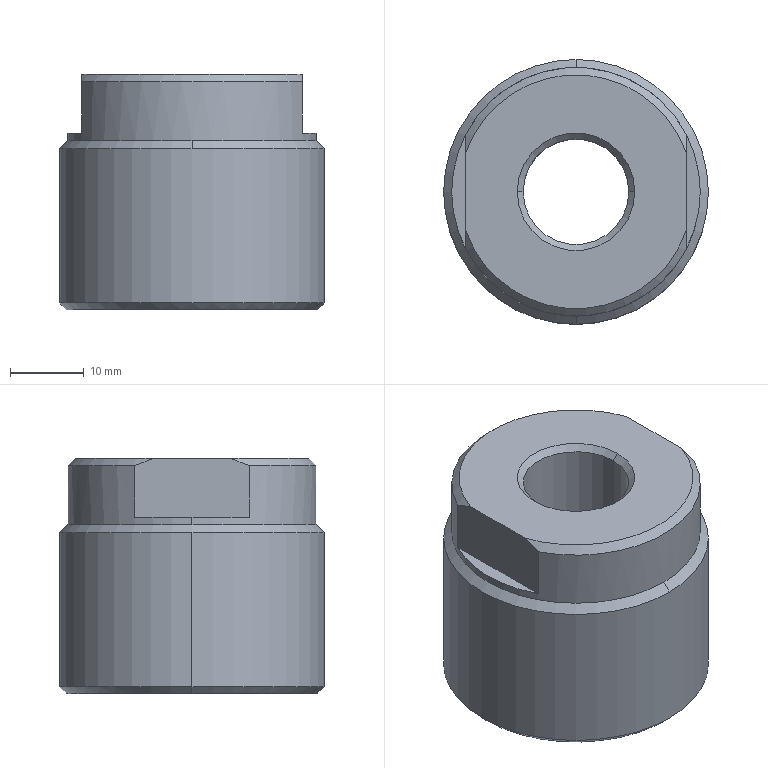Part | SolidWorks | features BaseBody 1 | 1 solid | 25 faces | box 36 x 36 x 32 mm | volume 25281 mm3 | cone 10 | cylinder 8 | plane 7 | commonest cylinder face diameters 14.376 x2 16.5 x2 33.8 x2 36 x2
STEP:
#1=CARTESIAN_POINT('',(18.,0.,0.92));
#2=VERTEX_POINT('',#1);
#3=CARTESIAN_POINT('',(-18.,0.,0.92));
#4=VERTEX_POINT('',#3);
#5=CARTESIAN_POINT('',(0.,0.,0.92));
#6=DIRECTION('',(0.,0.,1.));
#7=DIRECTION('',(1.,0.,0.));
#8=AXIS2_PLACEMENT_3D('',#5,#6,#7);
#9=CIRCLE('',#8,18.);
#10=EDGE_CURVE('',#2,#4,#9,.T.);
#11=ORIENTED_EDGE('',*,*,#10,.T.);
#12=CARTESIAN_POINT('',(-18.,0.,21.9));
#13=VERTEX_POINT('',#12);
#14=CARTESIAN_POINT('',(-18.,0.,0.));
#15=DIRECTION('',(0.,0.,1.));
#16=VECTOR('',#15,1000.);
#17=LINE('',#14,#16);
#18=EDGE_CURVE('',#4,#13,#17,.T.);
#19=ORIENTED_EDGE('',*,*,#18,.T.);
#20=CARTESIAN_POINT('',(0.,18.,21.9));
#21=VERTEX_POINT('',#20);
#22=CARTESIAN_POINT('',(0.,0.,21.9));
#23=DIRECTION('',(0.,0.,-1.));
#24=DIRECTION('',(1.,0.,0.));
#25=AXIS2_PLACEMENT_3D('',#22,#23,#24);
#26=CIRCLE('',#25,18.);
#27=EDGE_CURVE('',#13,#21,#26,.T.);
#28=ORIENTED_EDGE('',*,*,#27,.T.);
#29=CARTESIAN_POINT('',(18.,0.,21.9));
#30=VERTEX_POINT('',#29);
#31=CARTESIAN_POINT('',(0.,0.,21.9));
#32=DIRECTION('',(0.,0.,-1.));
#33=DIRECTION('',(1.,0.,0.));
#34=AXIS2_PLACEMENT_3D('',#31,#32,#33);
#35=CIRCLE('',#34,18.);
#36=EDGE_CURVE('',#21,#30,#35,.T.);
#37=ORIENTED_EDGE('',*,*,#36,.T.);
#38=CARTESIAN_POINT('',(18.,0.,0.));
#39=DIRECTION('',(0.,0.,1.));
#40=VECTOR('',#39,1000.);
#41=LINE('',#38,#40);
#42=EDGE_CURVE('',#2,#30,#41,.T.);
#43=ORIENTED_EDGE('',*,*,#42,.F.);
#44=EDGE_LOOP('',(#11,#19,#28,#37,#43));
#45=FACE_OUTER_BOUND('',#44,.T.);
#46=CARTESIAN_POINT('',(0.,0.,0.));
#47=DIRECTION('',(0.,0.,1.));
#48=DIRECTION('',(1.,0.,0.));
#49=AXIS2_PLACEMENT_3D('',#46,#47,#48);
#50=CYLINDRICAL_SURFACE('',#49,18.);
#51=ADVANCED_FACE('',(#45),#50,.T.);
#52=CARTESIAN_POINT('',(17.08,0.,0.));
#53=VERTEX_POINT('',#52);
#54=CARTESIAN_POINT('',(-17.08,0.,0.));
#55=VERTEX_POINT('',#54);
#56=CARTESIAN_POINT('',(0.,0.,0.));
#57=DIRECTION('',(0.,0.,1.));
#58=DIRECTION('',(1.,0.,0.));
#59=AXIS2_PLACEMENT_3D('',#56,#57,#58);
#60=CIRCLE('',#59,17.08);
#61=EDGE_CURVE('',#53,#55,#60,.T.);
#62=ORIENTED_EDGE('',*,*,#61,.T.);
#63=CARTESIAN_POINT('',(-18.,0.,0.92));
#64=DIRECTION('',(-0.7071,0.,0.7071));
#65=VECTOR('',#64,1000.);
#66=LINE('',#63,#65);
#67=EDGE_CURVE('',#55,#4,#66,.T.);
#68=ORIENTED_EDGE('',*,*,#67,.T.);
#69=ORIENTED_EDGE('',*,*,#10,.F.);
#70=CARTESIAN_POINT('',(18.,0.,0.92));
#71=DIRECTION('',(0.7071,0.,0.7071));
#72=VECTOR('',#71,1000.);
#73=LINE('',#70,#72);
#74=EDGE_CURVE('',#53,#2,#73,.T.);
#75=ORIENTED_EDGE('',*,*,#74,.F.);
#76=EDGE_LOOP('',(#62,#68,#69,#75));
#77=FACE_OUTER_BOUND('',#76,.T.);
#78=CARTESIAN_POINT('',(0.,0.,0.92));
#79=DIRECTION('',(0.,0.,1.));
#80=DIRECTION('',(1.,0.,0.));
#81=AXIS2_PLACEMENT_3D('',#78,#79,#80);
#82=CONICAL_SURFACE('',#81,18.,0.7854);
#83=ADVANCED_FACE('',(#77),#82,.T.);
#84=CARTESIAN_POINT('',(16.9,0.,23.));
#85=VERTEX_POINT('',#84);
#86=CARTESIAN_POINT('',(0.,-16.9,23.));
#87=VERTEX_POINT('',#86);
#88=CARTESIAN_POINT('',(0.,0.,23.));
#89=DIRECTION('',(0.,0.,-1.));
#90=DIRECTION('',(-1.,0.,0.));
#91=AXIS2_PLACEMENT_3D('',#88,#89,#90);
#92=CIRCLE('',#91,16.9);
#93=EDGE_CURVE('',#85,#87,#92,.T.);
#94=ORIENTED_EDGE('',*,*,#93,.T.);
#95=CARTESIAN_POINT('',(0.,-18.,21.9));
#96=VERTEX_POINT('',#95);
#97=CARTESIAN_POINT('',(0.,-18.,21.9));
#98=DIRECTION('',(0.,-0.7071,-0.7071));
#99=VECTOR('',#98,1000.);
#100=LINE('',#97,#99);
#101=EDGE_CURVE('',#87,#96,#100,.T.);
#102=ORIENTED_EDGE('',*,*,#101,.T.);
#103=CARTESIAN_POINT('',(0.,0.,21.9));
#104=DIRECTION('',(0.,0.,-1.));
#105=DIRECTION('',(1.,0.,0.));
#106=AXIS2_PLACEMENT_3D('',#103,#104,#105);
#107=CIRCLE('',#106,18.);
#108=EDGE_CURVE('',#30,#96,#107,.T.);
#109=ORIENTED_EDGE('',*,*,#108,.F.);
#110=ORIENTED_EDGE('',*,*,#36,.F.);
#111=CARTESIAN_POINT('',(0.,16.9,23.));
#112=VERTEX_POINT('',#111);
#113=CARTESIAN_POINT('',(0.,18.,21.9));
#114=DIRECTION('',(0.,0.7071,-0.7071));
#115=VECTOR('',#114,1000.);
#116=LINE('',#113,#115);
#117=EDGE_CURVE('',#112,#21,#116,.T.);
#118=ORIENTED_EDGE('',*,*,#117,.F.);
#119=CARTESIAN_POINT('',(0.,0.,23.));
#120=DIRECTION('',(0.,0.,-1.));
#121=DIRECTION('',(-1.,0.,0.));
#122=AXIS2_PLACEMENT_3D('',#119,#120,#121);
#123=CIRCLE('',#122,16.9);
#124=EDGE_CURVE('',#112,#85,#123,.T.);
#125=ORIENTED_EDGE('',*,*,#124,.T.);
#126=EDGE_LOOP('',(#94,#102,#109,#110,#118,#125));
#127=FACE_OUTER_BOUND('',#126,.T.);
#128=CARTESIAN_POINT('',(0.,0.,21.9));
#129=DIRECTION('',(0.,0.,-1.));
#130=DIRECTION('',(0.,1.,0.));
#131=AXIS2_PLACEMENT_3D('',#128,#129,#130);
#132=CONICAL_SURFACE('',#131,18.,0.7854);
#133=ADVANCED_FACE('',(#127),#132,.T.);
#134=CARTESIAN_POINT('',(-16.9,0.,23.));
#135=VERTEX_POINT('',#134);
#136=CARTESIAN_POINT('',(0.,0.,23.));
#137=DIRECTION('',(0.,0.,-1.));
#138=DIRECTION('',(-1.,0.,0.));
#139=AXIS2_PLACEMENT_3D('',#136,#137,#138);
#140=CIRCLE('',#139,16.9);
#141=EDGE_CURVE('',#135,#112,#140,.T.);
#142=ORIENTED_EDGE('',*,*,#141,.F.);
#143=CARTESIAN_POINT('',(-16.9,0.,24.));
#144=VERTEX_POINT('',#143);
#145=CARTESIAN_POINT('',(-16.9,0.,0.));
#146=DIRECTION('',(0.,0.,1.));
#147=VECTOR('',#146,1000.);
#148=LINE('',#145,#147);
#149=EDGE_CURVE('',#135,#144,#148,.T.);
#150=ORIENTED_EDGE('',*,*,#149,.T.);
#151=CARTESIAN_POINT('',(-15.,7.785,24.));
#152=VERTEX_POINT('',#151);
#153=CARTESIAN_POINT('',(0.,0.,24.));
#154=DIRECTION('',(0.,0.,-1.));
#155=DIRECTION('',(1.,0.,0.));
#156=AXIS2_PLACEMENT_3D('',#153,#154,#155);
#157=CIRCLE('',#156,16.9);
#158=EDGE_CURVE('',#144,#152,#157,.T.);
#159=ORIENTED_EDGE('',*,*,#158,.T.);
#160=CARTESIAN_POINT('',(-15.,7.785,31.));
#161=VERTEX_POINT('',#160);
#162=CARTESIAN_POINT('',(-15.,7.785,0.));
#163=DIRECTION('',(0.,0.,1.));
#164=VECTOR('',#163,1000.);
#165=LINE('',#162,#164);
#166=EDGE_CURVE('',#152,#161,#165,.T.);
#167=ORIENTED_EDGE('',*,*,#166,.T.);
#168=CARTESIAN_POINT('',(15.,7.785,31.));
#169=VERTEX_POINT('',#168);
#170=CARTESIAN_POINT('',(0.,0.,31.));
#171=DIRECTION('',(0.,0.,-1.));
#172=DIRECTION('',(1.,0.,0.));
#173=AXIS2_PLACEMENT_3D('',#170,#171,#172);
#174=CIRCLE('',#173,16.9);
#175=EDGE_CURVE('',#161,#169,#174,.T.);
#176=ORIENTED_EDGE('',*,*,#175,.T.);
#177=CARTESIAN_POINT('',(15.,7.785,24.));
#178=VERTEX_POINT('',#177);
#179=CARTESIAN_POINT('',(15.,7.785,0.));
#180=DIRECTION('',(0.,0.,-1.));
#181=VECTOR('',#180,1000.);
#182=LINE('',#179,#181);
#183=EDGE_CURVE('',#169,#178,#182,.T.);
#184=ORIENTED_EDGE('',*,*,#183,.T.);
#185=CARTESIAN_POINT('',(16.9,0.,24.));
#186=VERTEX_POINT('',#185);
#187=CARTESIAN_POINT('',(0.,0.,24.));
#188=DIRECTION('',(0.,0.,-1.));
#189=DIRECTION('',(1.,0.,0.));
#190=AXIS2_PLACEMENT_3D('',#187,#188,#189);
#191=CIRCLE('',#190,16.9);
#192=EDGE_CURVE('',#178,#186,#191,.T.);
#193=ORIENTED_EDGE('',*,*,#192,.T.);
#194=CARTESIAN_POINT('',(16.9,0.,0.));
#195=DIRECTION('',(0.,0.,1.));
#196=VECTOR('',#195,1000.);
#197=LINE('',#194,#196);
#198=EDGE_CURVE('',#85,#186,#197,.T.);
#199=ORIENTED_EDGE('',*,*,#198,.F.);
#200=ORIENTED_EDGE('',*,*,#124,.F.);
#201=EDGE_LOOP('',(#142,#150,#159,#167,#176,#184,#193,#199,#200));
#202=FACE_OUTER_BOUND('',#201,.T.);
#203=CARTESIAN_POINT('',(0.,0.,0.));
#204=DIRECTION('',(0.,0.,1.));
#205=DIRECTION('',(1.,0.,0.));
#206=AXIS2_PLACEMENT_3D('',#203,#204,#205);
#207=CYLINDRICAL_SURFACE('',#206,16.9);
#208=ADVANCED_FACE('',(#202),#207,.T.);
#209=CARTESIAN_POINT('',(8.25,0.,0.6));
#210=VERTEX_POINT('',#209);
#211=CARTESIAN_POINT('',(-8.25,0.,0.6));
#212=VERTEX_POINT('',#211);
#213=CARTESIAN_POINT('',(0.,0.,0.6));
#214=DIRECTION('',(0.,0.,-1.));
#215=DIRECTION('',(-1.,0.,0.));
#216=AXIS2_PLACEMENT_3D('',#213,#214,#215);
#217=CIRCLE('',#216,8.25);
#218=EDGE_CURVE('',#210,#212,#217,.T.);
#219=ORIENTED_EDGE('',*,*,#218,.F.);
#220=CARTESIAN_POINT('',(8.85,0.,0.));
#221=VERTEX_POINT('',#220);
#222=CARTESIAN_POINT('',(8.85,0.,0.));
#223=DIRECTION('',(0.7071,0.,-0.7071));
#224=VECTOR('',#223,1000.);
#225=LINE('',#222,#224);
#226=EDGE_CURVE('',#210,#221,#225,.T.);
#227=ORIENTED_EDGE('',*,*,#226,.T.);
#228=CARTESIAN_POINT('',(-8.85,0.,0.));
#229=VERTEX_POINT('',#228);
#230=CARTESIAN_POINT('',(0.,0.,0.));
#231=DIRECTION('',(0.,0.,1.));
#232=DIRECTION('',(-1.,0.,0.));
#233=AXIS2_PLACEMENT_3D('',#230,#231,#232);
#234=CIRCLE('',#233,8.85);
#235=EDGE_CURVE('',#229,#221,#234,.T.);
#236=ORIENTED_EDGE('',*,*,#235,.F.);
#237=CARTESIAN_POINT('',(-8.85,0.,0.));
#238=DIRECTION('',(-0.7071,0.,-0.7071));
#239=VECTOR('',#238,1000.);
#240=LINE('',#237,#239);
#241=EDGE_CURVE('',#212,#229,#240,.T.);
#242=ORIENTED_EDGE('',*,*,#241,.F.);
#243=EDGE_LOOP('',(#219,#227,#236,#242));
#244=FACE_OUTER_BOUND('',#243,.T.);
#245=CARTESIAN_POINT('',(0.,0.,0.));
#246=DIRECTION('',(0.,0.,-1.));
#247=DIRECTION('',(-1.,0.,0.));
#248=AXIS2_PLACEMENT_3D('',#245,#246,#247);
#249=CONICAL_SURFACE('',#248,8.85,0.7854);
#250=ADVANCED_FACE('',(#244),#249,.F.);
#251=ORIENTED_EDGE('',*,*,#218,.T.);
#252=CARTESIAN_POINT('',(-8.25,0.,10.));
#253=VERTEX_POINT('',#252);
#254=CARTESIAN_POINT('',(-8.25,0.,0.));
#255=DIRECTION('',(0.,0.,1.));
#256=VECTOR('',#255,1000.);
#257=LINE('',#254,#256);
#258=EDGE_CURVE('',#212,#253,#257,.T.);
#259=ORIENTED_EDGE('',*,*,#258,.T.);
#260=CARTESIAN_POINT('',(8.25,0.,10.));
#261=VERTEX_POINT('',#260);
#262=CARTESIAN_POINT('',(0.,0.,10.));
#263=DIRECTION('',(0.,0.,-1.));
#264=DIRECTION('',(1.,0.,0.));
#265=AXIS2_PLACEMENT_3D('',#262,#263,#264);
#266=CIRCLE('',#265,8.25);
#267=EDGE_CURVE('',#261,#253,#266,.T.);
#268=ORIENTED_EDGE('',*,*,#267,.F.);
#269=CARTESIAN_POINT('',(8.25,0.,0.));
#270=DIRECTION('',(0.,0.,1.));
#271=VECTOR('',#270,1000.);
#272=LINE('',#269,#271);
#273=EDGE_CURVE('',#210,#261,#272,.T.);
#274=ORIENTED_EDGE('',*,*,#273,.F.);
#275=EDGE_LOOP('',(#251,#259,#268,#274));
#276=FACE_OUTER_BOUND('',#275,.T.);
#277=CARTESIAN_POINT('',(0.,0.,0.));
#278=DIRECTION('',(0.,0.,1.));
#279=DIRECTION('',(1.,0.,0.));
#280=AXIS2_PLACEMENT_3D('',#277,#278,#279);
#281=CYLINDRICAL_SURFACE('',#280,8.25);
#282=ADVANCED_FACE('',(#276),#281,.F.);
#283=CARTESIAN_POINT('',(-7.188,0.,31.188));
#284=VERTEX_POINT('',#283);
#285=CARTESIAN_POINT('',(7.188,0.,31.188));
#286=VERTEX_POINT('',#285);
#287=CARTESIAN_POINT('',(0.,0.,31.188));
#288=DIRECTION('',(0.,0.,1.));
#289=DIRECTION('',(1.,0.,0.));
#290=AXIS2_PLACEMENT_3D('',#287,#288,#289);
#291=CIRCLE('',#290,7.188);
#292=EDGE_CURVE('',#284,#286,#291,.T.);
#293=ORIENTED_EDGE('',*,*,#292,.F.);
#294=CARTESIAN_POINT('',(-8.,0.,32.));
#295=VERTEX_POINT('',#294);
#296=CARTESIAN_POINT('',(-8.,0.,32.));
#297=DIRECTION('',(-0.7071,0.,0.7071));
#298=VECTOR('',#297,1000.);
#299=LINE('',#296,#298);
#300=EDGE_CURVE('',#284,#295,#299,.T.);
#301=ORIENTED_EDGE('',*,*,#300,.T.);
#302=CARTESIAN_POINT('',(8.,0.,32.));
#303=VERTEX_POINT('',#302);
#304=CARTESIAN_POINT('',(0.,0.,32.));
#305=DIRECTION('',(0.,0.,-1.));
#306=DIRECTION('',(1.,0.,0.));
#307=AXIS2_PLACEMENT_3D('',#304,#305,#306);
#308=CIRCLE('',#307,8.);
#309=EDGE_CURVE('',#303,#295,#308,.T.);
#310=ORIENTED_EDGE('',*,*,#309,.F.);
#311=CARTESIAN_POINT('',(8.,0.,32.));
#312=DIRECTION('',(0.7071,0.,0.7071));
#313=VECTOR('',#312,1000.);
#314=LINE('',#311,#313);
#315=EDGE_CURVE('',#286,#303,#314,.T.);
#316=ORIENTED_EDGE('',*,*,#315,.F.);
#317=EDGE_LOOP('',(#293,#301,#310,#316));
#318=FACE_OUTER_BOUND('',#317,.T.);
#319=CARTESIAN_POINT('',(0.,0.,32.));
#320=DIRECTION('',(0.,0.,1.));
#321=DIRECTION('',(1.,0.,0.));
#322=AXIS2_PLACEMENT_3D('',#319,#320,#321);
#323=CONICAL_SURFACE('',#322,8.,0.7854);
#324=ADVANCED_FACE('',(#318),#323,.F.);
#325=CARTESIAN_POINT('',(-7.188,0.,10.));
#326=VERTEX_POINT('',#325);
#327=CARTESIAN_POINT('',(7.188,0.,10.));
#328=VERTEX_POINT('',#327);
#329=CARTESIAN_POINT('',(0.,0.,10.));
#330=DIRECTION('',(0.,0.,1.));
#331=DIRECTION('',(1.,0.,0.));
#332=AXIS2_PLACEMENT_3D('',#329,#330,#331);
#333=CIRCLE('',#332,7.188);
#334=EDGE_CURVE('',#326,#328,#333,.T.);
#335=ORIENTED_EDGE('',*,*,#334,.F.);
#336=CARTESIAN_POINT('',(-7.188,0.,0.));
#337=DIRECTION('',(0.,0.,1.));
#338=VECTOR('',#337,1000.);
#339=LINE('',#336,#338);
#340=EDGE_CURVE('',#326,#284,#339,.T.);
#341=ORIENTED_EDGE('',*,*,#340,.T.);
#342=ORIENTED_EDGE('',*,*,#292,.T.);
#343=CARTESIAN_POINT('',(7.188,0.,0.));
#344=DIRECTION('',(0.,0.,1.));
#345=VECTOR('',#344,1000.);
#346=LINE('',#343,#345);
#347=EDGE_CURVE('',#328,#286,#346,.T.);
#348=ORIENTED_EDGE('',*,*,#347,.F.);
#349=EDGE_LOOP('',(#335,#341,#342,#348));
#350=FACE_OUTER_BOUND('',#349,.T.);
#351=CARTESIAN_POINT('',(0.,0.,0.));
#352=DIRECTION('',(0.,0.,1.));
#353=DIRECTION('',(1.,0.,0.));
#354=AXIS2_PLACEMENT_3D('',#351,#352,#353);
#355=CYLINDRICAL_SURFACE('',#354,7.188);
#356=ADVANCED_FACE('',(#350),#355,.F.);
#357=ORIENTED_EDGE('',*,*,#18,.F.);
#358=CARTESIAN_POINT('',(0.,0.,0.92));
#359=DIRECTION('',(0.,0.,1.));
#360=DIRECTION('',(1.,0.,0.));
#361=AXIS2_PLACEMENT_3D('',#358,#359,#360);
#362=CIRCLE('',#361,18.);
#363=EDGE_CURVE('',#4,#2,#362,.T.);
#364=ORIENTED_EDGE('',*,*,#363,.T.);
#365=ORIENTED_EDGE('',*,*,#42,.T.);
#366=ORIENTED_EDGE('',*,*,#108,.T.);
#367=CARTESIAN_POINT('',(0.,0.,21.9));
#368=DIRECTION('',(0.,0.,-1.));
#369=DIRECTION('',(1.,0.,0.));
#370=AXIS2_PLACEMENT_3D('',#367,#368,#369);
#371=CIRCLE('',#370,18.);
#372=EDGE_CURVE('',#96,#13,#371,.T.);
#373=ORIENTED_EDGE('',*,*,#372,.T.);
#374=EDGE_LOOP('',(#357,#364,#365,#366,#373));
#375=FACE_OUTER_BOUND('',#374,.T.);
#376=CARTESIAN_POINT('',(0.,0.,0.));
#377=DIRECTION('',(0.,0.,1.));
#378=DIRECTION('',(1.,0.,0.));
#379=AXIS2_PLACEMENT_3D('',#376,#377,#378);
#380=CYLINDRICAL_SURFACE('',#379,18.);
#381=ADVANCED_FACE('',(#375),#380,.T.);
#382=ORIENTED_EDGE('',*,*,#67,.F.);
#383=CARTESIAN_POINT('',(0.,0.,0.));
#384=DIRECTION('',(0.,0.,1.));
#385=DIRECTION('',(1.,0.,0.));
#386=AXIS2_PLACEMENT_3D('',#383,#384,#385);
#387=CIRCLE('',#386,17.08);
#388=EDGE_CURVE('',#55,#53,#387,.T.);
#389=ORIENTED_EDGE('',*,*,#388,.T.);
#390=ORIENTED_EDGE('',*,*,#74,.T.);
#391=ORIENTED_EDGE('',*,*,#363,.F.);
#392=EDGE_LOOP('',(#382,#389,#390,#391));
#393=FACE_OUTER_BOUND('',#392,.T.);
#394=CARTESIAN_POINT('',(0.,0.,0.92));
#395=DIRECTION('',(0.,0.,1.));
#396=DIRECTION('',(1.,0.,0.));
#397=AXIS2_PLACEMENT_3D('',#394,#395,#396);
#398=CONICAL_SURFACE('',#397,18.,0.7854);
#399=ADVANCED_FACE('',(#393),#398,.T.);
#400=ORIENTED_EDGE('',*,*,#101,.F.);
#401=CARTESIAN_POINT('',(0.,0.,23.));
#402=DIRECTION('',(0.,0.,-1.));
#403=DIRECTION('',(-1.,0.,0.));
#404=AXIS2_PLACEMENT_3D('',#401,#402,#403);
#405=CIRCLE('',#404,16.9);
#406=EDGE_CURVE('',#87,#135,#405,.T.);
#407=ORIENTED_EDGE('',*,*,#406,.T.);
#408=ORIENTED_EDGE('',*,*,#141,.T.);
#409=ORIENTED_EDGE('',*,*,#117,.T.);
#410=ORIENTED_EDGE('',*,*,#27,.F.);
#411=ORIENTED_EDGE('',*,*,#372,.F.);
#412=EDGE_LOOP('',(#400,#407,#408,#409,#410,#411));
#413=FACE_OUTER_BOUND('',#412,.T.);
#414=CARTESIAN_POINT('',(0.,0.,21.9));
#415=DIRECTION('',(0.,0.,-1.));
#416=DIRECTION('',(0.,1.,0.));
#417=AXIS2_PLACEMENT_3D('',#414,#415,#416);
#418=CONICAL_SURFACE('',#417,18.,0.7854);
#419=ADVANCED_FACE('',(#413),#418,.T.);
#420=ORIENTED_EDGE('',*,*,#235,.T.);
#421=CARTESIAN_POINT('',(0.,0.,0.));
#422=DIRECTION('',(0.,0.,1.));
#423=DIRECTION('',(-1.,0.,0.));
#424=AXIS2_PLACEMENT_3D('',#421,#422,#423);
#425=CIRCLE('',#424,8.85);
#426=EDGE_CURVE('',#221,#229,#425,.T.);
#427=ORIENTED_EDGE('',*,*,#426,.T.);
#428=EDGE_LOOP('',(#420,#427));
#429=FACE_BOUND('',#428,.T.);
#430=ORIENTED_EDGE('',*,*,#61,.F.);
#431=ORIENTED_EDGE('',*,*,#388,.F.);
#432=EDGE_LOOP('',(#430,#431));
#433=FACE_OUTER_BOUND('',#432,.T.);
#434=CARTESIAN_POINT('',(0.,8.85,0.));
#435=DIRECTION('',(0.,0.,-1.));
#436=DIRECTION('',(-1.,0.,0.));
#437=AXIS2_PLACEMENT_3D('',#434,#435,#436);
#438=PLANE('',#437);
#439=ADVANCED_FACE('',(#429,#433),#438,.T.);
#440=ORIENTED_EDGE('',*,*,#149,.F.);
#441=ORIENTED_EDGE('',*,*,#406,.F.);
#442=ORIENTED_EDGE('',*,*,#93,.F.);
#443=ORIENTED_EDGE('',*,*,#198,.T.);
#444=CARTESIAN_POINT('',(15.,-7.785,24.));
#445=VERTEX_POINT('',#444);
#446=CARTESIAN_POINT('',(0.,0.,24.));
#447=DIRECTION('',(0.,0.,-1.));
#448=DIRECTION('',(1.,0.,0.));
#449=AXIS2_PLACEMENT_3D('',#446,#447,#448);
#450=CIRCLE('',#449,16.9);
#451=EDGE_CURVE('',#186,#445,#450,.T.);
#452=ORIENTED_EDGE('',*,*,#451,.T.);
#453=CARTESIAN_POINT('',(15.,-7.785,31.));
#454=VERTEX_POINT('',#453);
#455=CARTESIAN_POINT('',(15.,-7.785,0.));
#456=DIRECTION('',(0.,0.,1.));
#457=VECTOR('',#456,1000.);
#458=LINE('',#455,#457);
#459=EDGE_CURVE('',#445,#454,#458,.T.);
#460=ORIENTED_EDGE('',*,*,#459,.T.);
#461=CARTESIAN_POINT('',(-15.,-7.785,31.));
#462=VERTEX_POINT('',#461);
#463=CARTESIAN_POINT('',(0.,0.,31.));
#464=DIRECTION('',(0.,0.,-1.));
#465=DIRECTION('',(1.,0.,0.));
#466=AXIS2_PLACEMENT_3D('',#463,#464,#465);
#467=CIRCLE('',#466,16.9);
#468=EDGE_CURVE('',#454,#462,#467,.T.);
#469=ORIENTED_EDGE('',*,*,#468,.T.);
#470=CARTESIAN_POINT('',(-15.,-7.785,24.));
#471=VERTEX_POINT('',#470);
#472=CARTESIAN_POINT('',(-15.,-7.785,0.));
#473=DIRECTION('',(0.,0.,-1.));
#474=VECTOR('',#473,1000.);
#475=LINE('',#472,#474);
#476=EDGE_CURVE('',#462,#471,#475,.T.);
#477=ORIENTED_EDGE('',*,*,#476,.T.);
#478=CARTESIAN_POINT('',(0.,0.,24.));
#479=DIRECTION('',(0.,0.,-1.));
#480=DIRECTION('',(1.,0.,0.));
#481=AXIS2_PLACEMENT_3D('',#478,#479,#480);
#482=CIRCLE('',#481,16.9);
#483=EDGE_CURVE('',#471,#144,#482,.T.);
#484=ORIENTED_EDGE('',*,*,#483,.T.);
#485=EDGE_LOOP('',(#440,#441,#442,#443,#452,#460,#469,#477,#484));
#486=FACE_OUTER_BOUND('',#485,.T.);
#487=CARTESIAN_POINT('',(0.,0.,0.));
#488=DIRECTION('',(0.,0.,1.));
#489=DIRECTION('',(1.,0.,0.));
#490=AXIS2_PLACEMENT_3D('',#487,#488,#489);
#491=CYLINDRICAL_SURFACE('',#490,16.9);
#492=ADVANCED_FACE('',(#486),#491,.T.);
#493=ORIENTED_EDGE('',*,*,#226,.F.);
#494=CARTESIAN_POINT('',(0.,0.,0.6));
#495=DIRECTION('',(0.,0.,-1.));
#496=DIRECTION('',(-1.,0.,0.));
#497=AXIS2_PLACEMENT_3D('',#494,#495,#496);
#498=CIRCLE('',#497,8.25);
#499=EDGE_CURVE('',#212,#210,#498,.T.);
#500=ORIENTED_EDGE('',*,*,#499,.F.);
#501=ORIENTED_EDGE('',*,*,#241,.T.);
#502=ORIENTED_EDGE('',*,*,#426,.F.);
#503=EDGE_LOOP('',(#493,#500,#501,#502));
#504=FACE_OUTER_BOUND('',#503,.T.);
#505=CARTESIAN_POINT('',(0.,0.,0.));
#506=DIRECTION('',(0.,0.,-1.));
#507=DIRECTION('',(-1.,0.,0.));
#508=AXIS2_PLACEMENT_3D('',#505,#506,#507);
#509=CONICAL_SURFACE('',#508,8.85,0.7854);
#510=ADVANCED_FACE('',(#504),#509,.F.);
#511=CARTESIAN_POINT('',(-15.,30.,24.));
#512=DIRECTION('',(0.,1.,0.));
#513=VECTOR('',#512,1000.);
#514=LINE('',#511,#513);
#515=EDGE_CURVE('',#471,#152,#514,.T.);
#516=ORIENTED_EDGE('',*,*,#515,.T.);
#517=ORIENTED_EDGE('',*,*,#158,.F.);
#518=ORIENTED_EDGE('',*,*,#483,.F.);
#519=EDGE_LOOP('',(#516,#517,#518));
#520=FACE_OUTER_BOUND('',#519,.T.);
#521=CARTESIAN_POINT('',(-15.,30.,24.));
#522=DIRECTION('',(0.,0.,1.));
#523=DIRECTION('',(1.,0.,0.));
#524=AXIS2_PLACEMENT_3D('',#521,#522,#523);
#525=PLANE('',#524);
#526=ADVANCED_FACE('',(#520),#525,.T.);
#527=CARTESIAN_POINT('',(-15.,5.274,32.));
#528=VERTEX_POINT('',#527);
#529=CARTESIAN_POINT('',(-15.,5.274,32.));
#530=CARTESIAN_POINT('',(-15.,6.13,31.716));
#531=CARTESIAN_POINT('',(-15.,6.966,31.378));
#532=CARTESIAN_POINT('',(-15.,7.785,31.));
#533=B_SPLINE_CURVE_WITH_KNOTS('',3,(#529,#530,#531,#532),.UNSPECIFIED.,.F.,.F.,(4,4),(0.,0.002703),.UNSPECIFIED.);
#534=EDGE_CURVE('',#528,#161,#533,.T.);
#535=ORIENTED_EDGE('',*,*,#534,.T.);
#536=ORIENTED_EDGE('',*,*,#166,.F.);
#537=ORIENTED_EDGE('',*,*,#515,.F.);
#538=ORIENTED_EDGE('',*,*,#476,.F.);
#539=CARTESIAN_POINT('',(-15.,-5.274,32.));
#540=VERTEX_POINT('',#539);
#541=CARTESIAN_POINT('',(-15.,-7.785,31.));
#542=CARTESIAN_POINT('',(-15.,-6.966,31.378));
#543=CARTESIAN_POINT('',(-15.,-6.13,31.716));
#544=CARTESIAN_POINT('',(-15.,-5.274,32.));
#545=B_SPLINE_CURVE_WITH_KNOTS('',3,(#541,#542,#543,#544),.UNSPECIFIED.,.F.,.F.,(4,4),(0.,0.002703),.UNSPECIFIED.);
#546=EDGE_CURVE('',#462,#540,#545,.T.);
#547=ORIENTED_EDGE('',*,*,#546,.T.);
#548=CARTESIAN_POINT('',(-15.,30.,32.));
#549=DIRECTION('',(0.,1.,0.));
#550=VECTOR('',#549,1000.);
#551=LINE('',#548,#550);
#552=EDGE_CURVE('',#540,#528,#551,.T.);
#553=ORIENTED_EDGE('',*,*,#552,.T.);
#554=EDGE_LOOP('',(#535,#536,#537,#538,#547,#553));
#555=FACE_OUTER_BOUND('',#554,.T.);
#556=CARTESIAN_POINT('',(-15.,30.,39.));
#557=DIRECTION('',(-1.,0.,0.));
#558=DIRECTION('',(0.,0.,1.));
#559=AXIS2_PLACEMENT_3D('',#556,#557,#558);
#560=PLANE('',#559);
#561=ADVANCED_FACE('',(#555),#560,.T.);
#562=CARTESIAN_POINT('',(15.,-5.274,32.));
#563=VERTEX_POINT('',#562);
#564=CARTESIAN_POINT('',(0.,0.,32.));
#565=DIRECTION('',(0.,0.,-1.));
#566=DIRECTION('',(-1.,0.,0.));
#567=AXIS2_PLACEMENT_3D('',#564,#565,#566);
#568=CIRCLE('',#567,15.9);
#569=EDGE_CURVE('',#563,#540,#568,.T.);
#570=ORIENTED_EDGE('',*,*,#569,.T.);
#571=ORIENTED_EDGE('',*,*,#546,.F.);
#572=ORIENTED_EDGE('',*,*,#468,.F.);
#573=CARTESIAN_POINT('',(15.,-7.785,31.));
#574=CARTESIAN_POINT('',(15.,-6.966,31.378));
#575=CARTESIAN_POINT('',(15.,-6.13,31.716));
#576=CARTESIAN_POINT('',(15.,-5.274,32.));
#577=B_SPLINE_CURVE_WITH_KNOTS('',3,(#573,#574,#575,#576),.UNSPECIFIED.,.F.,.F.,(4,4),(0.,0.002703),.UNSPECIFIED.);
#578=EDGE_CURVE('',#454,#563,#577,.T.);
#579=ORIENTED_EDGE('',*,*,#578,.T.);
#580=EDGE_LOOP('',(#570,#571,#572,#579));
#581=FACE_OUTER_BOUND('',#580,.T.);
#582=CARTESIAN_POINT('',(0.,0.,31.));
#583=DIRECTION('',(0.,0.,-1.));
#584=DIRECTION('',(-1.,0.,0.));
#585=AXIS2_PLACEMENT_3D('',#582,#583,#584);
#586=CONICAL_SURFACE('',#585,16.9,0.7854);
#587=ADVANCED_FACE('',(#581),#586,.T.);
#588=ORIENTED_EDGE('',*,*,#578,.F.);
#589=ORIENTED_EDGE('',*,*,#459,.F.);
#590=CARTESIAN_POINT('',(15.,30.,24.));
#591=DIRECTION('',(0.,1.,0.));
#592=VECTOR('',#591,1000.);
#593=LINE('',#590,#592);
#594=EDGE_CURVE('',#445,#178,#593,.T.);
#595=ORIENTED_EDGE('',*,*,#594,.T.);
#596=ORIENTED_EDGE('',*,*,#183,.F.);
#597=CARTESIAN_POINT('',(15.,5.274,32.));
#598=VERTEX_POINT('',#597);
#599=CARTESIAN_POINT('',(15.,7.785,31.));
#600=CARTESIAN_POINT('',(15.,6.966,31.378));
#601=CARTESIAN_POINT('',(15.,6.13,31.716));
#602=CARTESIAN_POINT('',(15.,5.274,32.));
#603=B_SPLINE_CURVE_WITH_KNOTS('',3,(#599,#600,#601,#602),.UNSPECIFIED.,.F.,.F.,(4,4),(0.,0.002703),.UNSPECIFIED.);
#604=EDGE_CURVE('',#169,#598,#603,.T.);
#605=ORIENTED_EDGE('',*,*,#604,.T.);
#606=CARTESIAN_POINT('',(15.,30.,32.));
#607=DIRECTION('',(0.,-1.,0.));
#608=VECTOR('',#607,1000.);
#609=LINE('',#606,#608);
#610=EDGE_CURVE('',#598,#563,#609,.T.);
#611=ORIENTED_EDGE('',*,*,#610,.T.);
#612=EDGE_LOOP('',(#588,#589,#595,#596,#605,#611));
#613=FACE_OUTER_BOUND('',#612,.T.);
#614=CARTESIAN_POINT('',(15.,30.,24.));
#615=DIRECTION('',(1.,0.,0.));
#616=DIRECTION('',(0.,0.,-1.));
#617=AXIS2_PLACEMENT_3D('',#614,#615,#616);
#618=PLANE('',#617);
#619=ADVANCED_FACE('',(#613),#618,.T.);
#620=ORIENTED_EDGE('',*,*,#594,.F.);
#621=ORIENTED_EDGE('',*,*,#451,.F.);
#622=ORIENTED_EDGE('',*,*,#192,.F.);
#623=EDGE_LOOP('',(#620,#621,#622));
#624=FACE_OUTER_BOUND('',#623,.T.);
#625=CARTESIAN_POINT('',(25.,30.,24.));
#626=DIRECTION('',(0.,0.,1.));
#627=DIRECTION('',(1.,0.,0.));
#628=AXIS2_PLACEMENT_3D('',#625,#626,#627);
#629=PLANE('',#628);
#630=ADVANCED_FACE('',(#624),#629,.T.);
#631=CARTESIAN_POINT('',(0.,0.,32.));
#632=DIRECTION('',(0.,0.,-1.));
#633=DIRECTION('',(-1.,0.,0.));
#634=AXIS2_PLACEMENT_3D('',#631,#632,#633);
#635=CIRCLE('',#634,15.9);
#636=EDGE_CURVE('',#528,#598,#635,.T.);
#637=ORIENTED_EDGE('',*,*,#636,.T.);
#638=ORIENTED_EDGE('',*,*,#604,.F.);
#639=ORIENTED_EDGE('',*,*,#175,.F.);
#640=ORIENTED_EDGE('',*,*,#534,.F.);
#641=EDGE_LOOP('',(#637,#638,#639,#640));
#642=FACE_OUTER_BOUND('',#641,.T.);
#643=CARTESIAN_POINT('',(0.,0.,31.));
#644=DIRECTION('',(0.,0.,-1.));
#645=DIRECTION('',(-1.,0.,0.));
#646=AXIS2_PLACEMENT_3D('',#643,#644,#645);
#647=CONICAL_SURFACE('',#646,16.9,0.7854);
#648=ADVANCED_FACE('',(#642),#647,.T.);
#649=ORIENTED_EDGE('',*,*,#258,.F.);
#650=ORIENTED_EDGE('',*,*,#499,.T.);
#651=ORIENTED_EDGE('',*,*,#273,.T.);
#652=CARTESIAN_POINT('',(0.,0.,10.));
#653=DIRECTION('',(0.,0.,-1.));
#654=DIRECTION('',(1.,0.,0.));
#655=AXIS2_PLACEMENT_3D('',#652,#653,#654);
#656=CIRCLE('',#655,8.25);
#657=EDGE_CURVE('',#253,#261,#656,.T.);
#658=ORIENTED_EDGE('',*,*,#657,.F.);
#659=EDGE_LOOP('',(#649,#650,#651,#658));
#660=FACE_OUTER_BOUND('',#659,.T.);
#661=CARTESIAN_POINT('',(0.,0.,0.));
#662=DIRECTION('',(0.,0.,1.));
#663=DIRECTION('',(1.,0.,0.));
#664=AXIS2_PLACEMENT_3D('',#661,#662,#663);
#665=CYLINDRICAL_SURFACE('',#664,8.25);
#666=ADVANCED_FACE('',(#660),#665,.F.);
#667=ORIENTED_EDGE('',*,*,#636,.F.);
#668=ORIENTED_EDGE('',*,*,#552,.F.);
#669=ORIENTED_EDGE('',*,*,#569,.F.);
#670=ORIENTED_EDGE('',*,*,#610,.F.);
#671=EDGE_LOOP('',(#667,#668,#669,#670));
#672=FACE_OUTER_BOUND('',#671,.T.);
#673=ORIENTED_EDGE('',*,*,#309,.T.);
#674=CARTESIAN_POINT('',(0.,0.,32.));
#675=DIRECTION('',(0.,0.,-1.));
#676=DIRECTION('',(1.,0.,0.));
#677=AXIS2_PLACEMENT_3D('',#674,#675,#676);
#678=CIRCLE('',#677,8.);
#679=EDGE_CURVE('',#295,#303,#678,.T.);
#680=ORIENTED_EDGE('',*,*,#679,.T.);
#681=EDGE_LOOP('',(#673,#680));
#682=FACE_BOUND('',#681,.T.);
#683=CARTESIAN_POINT('',(0.,15.9,32.));
#684=DIRECTION('',(0.,0.,1.));
#685=DIRECTION('',(1.,0.,0.));
#686=AXIS2_PLACEMENT_3D('',#683,#684,#685);
#687=PLANE('',#686);
#688=ADVANCED_FACE('',(#672,#682),#687,.T.);
#689=CARTESIAN_POINT('',(0.,0.,10.));
#690=DIRECTION('',(0.,0.,1.));
#691=DIRECTION('',(1.,0.,0.));
#692=AXIS2_PLACEMENT_3D('',#689,#690,#691);
#693=CIRCLE('',#692,7.188);
#694=EDGE_CURVE('',#328,#326,#693,.T.);
#695=ORIENTED_EDGE('',*,*,#694,.T.);
#696=ORIENTED_EDGE('',*,*,#334,.T.);
#697=EDGE_LOOP('',(#695,#696));
#698=FACE_BOUND('',#697,.T.);
#699=ORIENTED_EDGE('',*,*,#267,.T.);
#700=ORIENTED_EDGE('',*,*,#657,.T.);
#701=EDGE_LOOP('',(#699,#700));
#702=FACE_OUTER_BOUND('',#701,.T.);
#703=CARTESIAN_POINT('',(0.,7.188,10.));
#704=DIRECTION('',(0.,0.,-1.));
#705=DIRECTION('',(-1.,0.,0.));
#706=AXIS2_PLACEMENT_3D('',#703,#704,#705);
#707=PLANE('',#706);
#708=ADVANCED_FACE('',(#698,#702),#707,.T.);
#709=ORIENTED_EDGE('',*,*,#300,.F.);
#710=CARTESIAN_POINT('',(0.,0.,31.188));
#711=DIRECTION('',(0.,0.,1.));
#712=DIRECTION('',(1.,0.,0.));
#713=AXIS2_PLACEMENT_3D('',#710,#711,#712);
#714=CIRCLE('',#713,7.188);
#715=EDGE_CURVE('',#286,#284,#714,.T.);
#716=ORIENTED_EDGE('',*,*,#715,.F.);
#717=ORIENTED_EDGE('',*,*,#315,.T.);
#718=ORIENTED_EDGE('',*,*,#679,.F.);
#719=EDGE_LOOP('',(#709,#716,#717,#718));
#720=FACE_OUTER_BOUND('',#719,.T.);
#721=CARTESIAN_POINT('',(0.,0.,32.));
#722=DIRECTION('',(0.,0.,1.));
#723=DIRECTION('',(1.,0.,0.));
#724=AXIS2_PLACEMENT_3D('',#721,#722,#723);
#725=CONICAL_SURFACE('',#724,8.,0.7854);
#726=ADVANCED_FACE('',(#720),#725,.F.);
#727=ORIENTED_EDGE('',*,*,#340,.F.);
#728=ORIENTED_EDGE('',*,*,#694,.F.);
#729=ORIENTED_EDGE('',*,*,#347,.T.);
#730=ORIENTED_EDGE('',*,*,#715,.T.);
#731=EDGE_LOOP('',(#727,#728,#729,#730));
#732=FACE_OUTER_BOUND('',#731,.T.);
#733=CARTESIAN_POINT('',(0.,0.,0.));
#734=DIRECTION('',(0.,0.,1.));
#735=DIRECTION('',(1.,0.,0.));
#736=AXIS2_PLACEMENT_3D('',#733,#734,#735);
#737=CYLINDRICAL_SURFACE('',#736,7.188);
#738=ADVANCED_FACE('',(#732),#737,.F.);
#739=CLOSED_SHELL('',(#51,#83,#133,#208,#250,#282,#324,#356,#381,#399,#419,#439,#492,#510,#526,#561,#587,#619,#630,#648,#666,#688,#708,#726,#738));
#740=MANIFOLD_SOLID_BREP('',#739);
#741=CARTESIAN_POINT('',(0.,0.,0.));
#742=DIRECTION('',(0.,0.,1.));
#743=DIRECTION('',(1.,0.,0.));
#744=AXIS2_PLACEMENT_3D('',#741,#742,#743);
#745=(LENGTH_UNIT()NAMED_UNIT(*)SI_UNIT(.MILLI.,.METRE.));
#746=UNCERTAINTY_MEASURE_WITH_UNIT(LENGTH_MEASURE(0.00001),#745,'','');
#747=(NAMED_UNIT(*)PLANE_ANGLE_UNIT()SI_UNIT($,.RADIAN.));
#748=(NAMED_UNIT(*)SI_UNIT($,.STERADIAN.)SOLID_ANGLE_UNIT());
#749=(GEOMETRIC_REPRESENTATION_CONTEXT(3)GLOBAL_UNCERTAINTY_ASSIGNED_CONTEXT((#746))GLOBAL_UNIT_ASSIGNED_CONTEXT((#745,#747,#748))REPRESENTATION_CONTEXT('',''));
#750=ADVANCED_BREP_SHAPE_REPRESENTATION('',(#740,#744),#749);